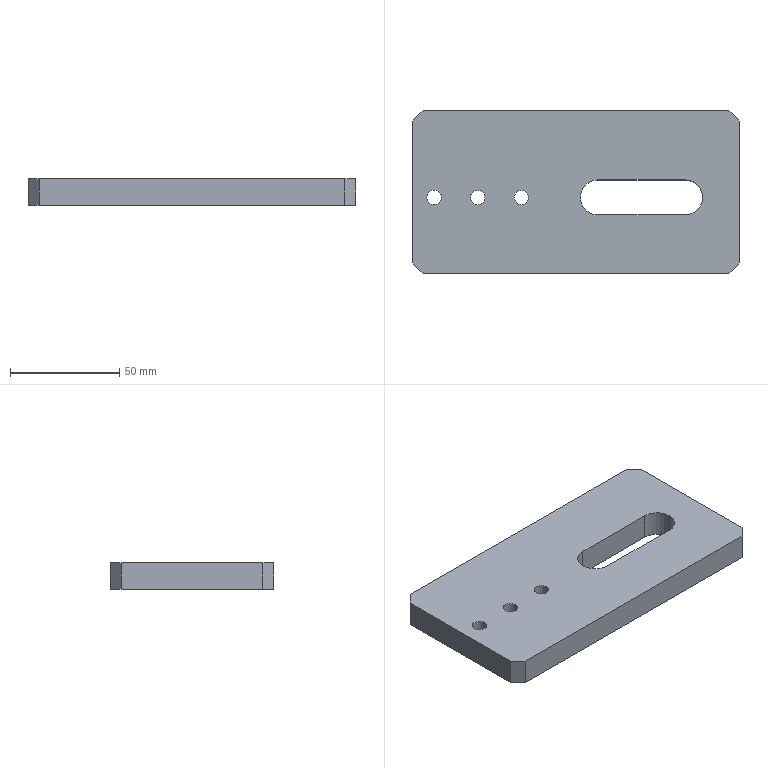Part | STEP file | Roller fixing plate | 1 solid | 30 faces | box 150 x 75 x 12 mm | volume 121835 mm3 | cylinder 15 | plane 15 | commonest cylinder face diameters 6.6 x6 11 x6 16 x3